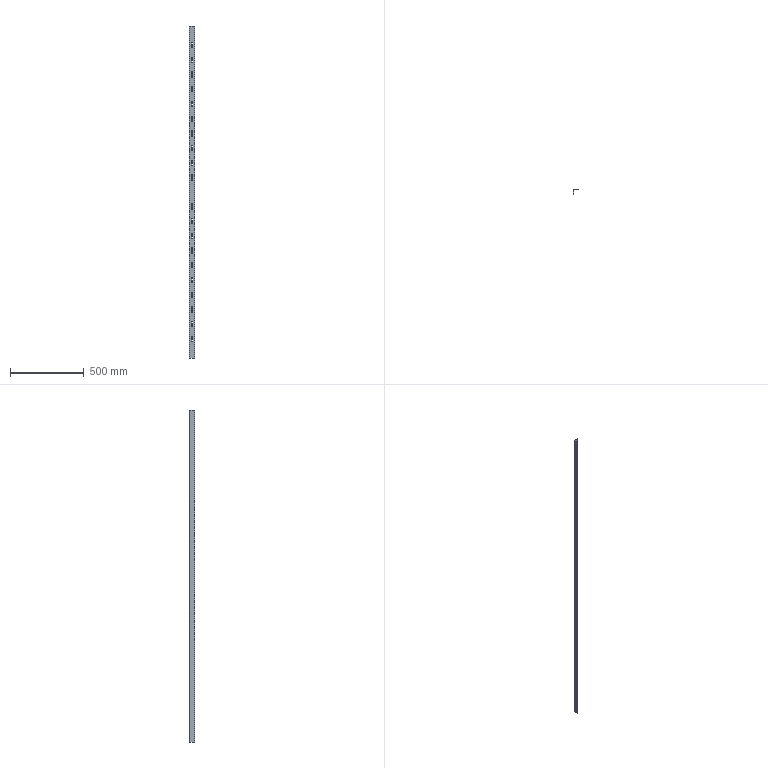Part | 1 solid | 114 faces | box 35 x 35 x 2256 mm | volume 223014 mm3 | cylinder 62 | plane 52 | commonest cylinder face diameters 6 x60 2 x1 5 x1